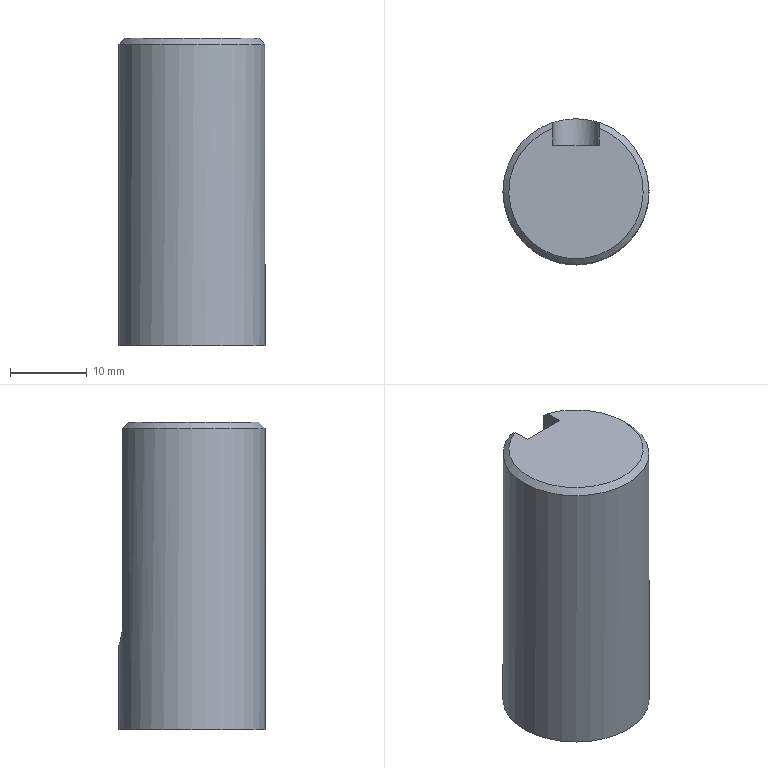Part | STEP file | Y2_SCZ_80_1.step 6 | 1 solid | 8 faces | box 19 x 19 x 40 mm | volume 10757 mm3 | plane 5 | cylinder 2 | cone 1 | commonest cylinder face diameters 6 x1 19 x1
STEP:
#1=CARTESIAN_POINT('',(0.,0.,0.));
#2=DIRECTION('',(0.,0.,1.));
#3=DIRECTION('',(1.,0.,0.));
#4=AXIS2_PLACEMENT_3D('',#1,#2,#3);
#5=CARTESIAN_POINT('',(3.,9.014,114.));
#6=VERTEX_POINT('',#5);
#7=CARTESIAN_POINT('',(3.,9.014,139.24));
#8=VERTEX_POINT('',#7);
#9=CARTESIAN_POINT('',(3.,9.014,100.));
#10=DIRECTION('',(0.,0.,1.));
#11=VECTOR('',#10,1.);
#12=LINE('',#9,#11);
#13=CARTESIAN_POINT('',(0.,0.,100.));
#14=DIRECTION('',(0.,0.,-1.));
#15=DIRECTION('',(-1.,0.,0.));
#16=AXIS2_PLACEMENT_3D('',#13,#14,#15);
#17=CYLINDRICAL_SURFACE('',#16,9.5);
#18=CARTESIAN_POINT('',(1.892,0.));
#19=DIRECTION('',(0.,-1.));
#20=VECTOR('',#19,1.);
#21=LINE('',#18,#20);
#22=(GEOMETRIC_REPRESENTATION_CONTEXT(2)PARAMETRIC_REPRESENTATION_CONTEXT()REPRESENTATION_CONTEXT('',''));
#23=DEFINITIONAL_REPRESENTATION('',(#21),#22);
#24=PCURVE('',#17,#23);
#25=CARTESIAN_POINT('',(3.,6.,140.));
#26=DIRECTION('',(1.,0.,0.));
#27=DIRECTION('',(0.,0.,-1.));
#28=AXIS2_PLACEMENT_3D('',#25,#26,#27);
#29=PLANE('',#28);
#30=CARTESIAN_POINT('',(40.,3.014));
#31=DIRECTION('',(-1.,0.));
#32=VECTOR('',#31,1.);
#33=LINE('',#30,#32);
#34=(GEOMETRIC_REPRESENTATION_CONTEXT(2)PARAMETRIC_REPRESENTATION_CONTEXT()REPRESENTATION_CONTEXT('',''));
#35=DEFINITIONAL_REPRESENTATION('',(#33),#34);
#36=PCURVE('',#29,#35);
#37=SURFACE_CURVE('',#12,(#24,#36),.PCURVE_S1.);
#38=EDGE_CURVE('',#6,#8,#37,.T.);
#39=ORIENTED_EDGE('',*,*,#38,.T.);
#40=CARTESIAN_POINT('',(-9.5,0.,139.24));
#41=VERTEX_POINT('',#40);
#42=CARTESIAN_POINT('',(0.,0.,139.24));
#43=DIRECTION('',(0.,0.,-1.));
#44=DIRECTION('',(-1.,0.,0.));
#45=AXIS2_PLACEMENT_3D('',#42,#43,#44);
#46=CIRCLE('',#45,9.5);
#47=CARTESIAN_POINT('',(0.,-39.24));
#48=DIRECTION('',(1.,0.));
#49=VECTOR('',#48,1.);
#50=LINE('',#47,#49);
#51=(GEOMETRIC_REPRESENTATION_CONTEXT(2)PARAMETRIC_REPRESENTATION_CONTEXT()REPRESENTATION_CONTEXT('',''));
#52=DEFINITIONAL_REPRESENTATION('',(#50),#51);
#53=PCURVE('',#17,#52);
#54=CARTESIAN_POINT('',(0.,0.,139.24));
#55=DIRECTION('',(0.,0.,-1.));
#56=DIRECTION('',(-1.,0.,0.));
#57=AXIS2_PLACEMENT_3D('',#54,#55,#56);
#58=CONICAL_SURFACE('',#57,9.5,0.7854);
#59=CARTESIAN_POINT('',(0.,0.));
#60=DIRECTION('',(1.,0.));
#61=VECTOR('',#60,1.);
#62=LINE('',#59,#61);
#63=(GEOMETRIC_REPRESENTATION_CONTEXT(2)PARAMETRIC_REPRESENTATION_CONTEXT()REPRESENTATION_CONTEXT('',''));
#64=DEFINITIONAL_REPRESENTATION('',(#62),#63);
#65=PCURVE('',#58,#64);
#66=SURFACE_CURVE('',#46,(#53,#65),.PCURVE_S1.);
#67=EDGE_CURVE('',#8,#41,#66,.T.);
#68=ORIENTED_EDGE('',*,*,#67,.T.);
#69=CARTESIAN_POINT('',(-9.5,0.,100.));
#70=VERTEX_POINT('',#69);
#71=CARTESIAN_POINT('',(-9.5,0.,139.24));
#72=CARTESIAN_POINT('',(-9.5,0.,100.));
#73=B_SPLINE_CURVE_WITH_KNOTS('',1,(#71,#72),.UNSPECIFIED.,.F.,.F.,(2,2),(-39.24,0.),.PIECEWISE_BEZIER_KNOTS.);
#74=CARTESIAN_POINT('',(6.283,0.));
#75=DIRECTION('',(0.,1.));
#76=VECTOR('',#75,1.);
#77=LINE('',#74,#76);
#78=(GEOMETRIC_REPRESENTATION_CONTEXT(2)PARAMETRIC_REPRESENTATION_CONTEXT()REPRESENTATION_CONTEXT('',''));
#79=DEFINITIONAL_REPRESENTATION('',(#77),#78);
#80=PCURVE('',#17,#79);
#81=CARTESIAN_POINT('',(0.,0.));
#82=DIRECTION('',(0.,1.));
#83=VECTOR('',#82,1.);
#84=LINE('',#81,#83);
#85=(GEOMETRIC_REPRESENTATION_CONTEXT(2)PARAMETRIC_REPRESENTATION_CONTEXT()REPRESENTATION_CONTEXT('',''));
#86=DEFINITIONAL_REPRESENTATION('',(#84),#85);
#87=PCURVE('',#17,#86);
#88=SEAM_CURVE('',#73,(#80,#87),.PCURVE_S1.);
#89=EDGE_CURVE('',#41,#70,#88,.T.);
#90=ORIENTED_EDGE('',*,*,#89,.T.);
#91=CARTESIAN_POINT('',(0.,0.,100.));
#92=DIRECTION('',(0.,0.,1.));
#93=DIRECTION('',(-1.,0.,0.));
#94=AXIS2_PLACEMENT_3D('',#91,#92,#93);
#95=CIRCLE('',#94,9.5);
#96=CARTESIAN_POINT('',(6.283,0.));
#97=DIRECTION('',(-1.,0.));
#98=VECTOR('',#97,1.);
#99=LINE('',#96,#98);
#100=(GEOMETRIC_REPRESENTATION_CONTEXT(2)PARAMETRIC_REPRESENTATION_CONTEXT()REPRESENTATION_CONTEXT('',''));
#101=DEFINITIONAL_REPRESENTATION('',(#99),#100);
#102=PCURVE('',#17,#101);
#103=CARTESIAN_POINT('',(0.,9.5,100.));
#104=DIRECTION('',(0.,0.,-1.));
#105=DIRECTION('',(-1.,0.,0.));
#106=AXIS2_PLACEMENT_3D('',#103,#104,#105);
#107=PLANE('',#106);
#108=CARTESIAN_POINT('',(9.5,-9.5));
#109=CARTESIAN_POINT('',(9.5,-25.954));
#110=CARTESIAN_POINT('',(-4.75,-17.727));
#111=CARTESIAN_POINT('',(-19.,-9.5));
#112=CARTESIAN_POINT('',(-4.75,-1.273));
#113=CARTESIAN_POINT('',(9.5,6.954));
#114=CARTESIAN_POINT('',(9.5,-9.5));
#115=(BOUNDED_CURVE()B_SPLINE_CURVE(2,(#108,#109,#110,#111,#112,#113,#114),.UNSPECIFIED.,.T.,.F.)B_SPLINE_CURVE_WITH_KNOTS((1,2,2,2,2,1),(-2.094,0.,2.094,4.189,6.283,8.378),.UNSPECIFIED.)CURVE()GEOMETRIC_REPRESENTATION_ITEM()RATIONAL_B_SPLINE_CURVE((1.,0.5,1.,0.5,1.,0.5,1.))REPRESENTATION_ITEM(''));
#116=(GEOMETRIC_REPRESENTATION_CONTEXT(2)PARAMETRIC_REPRESENTATION_CONTEXT()REPRESENTATION_CONTEXT('',''));
#117=DEFINITIONAL_REPRESENTATION('',(#115),#116);
#118=PCURVE('',#107,#117);
#119=SURFACE_CURVE('',#95,(#102,#118),.PCURVE_S1.);
#120=EDGE_CURVE('',#70,#70,#119,.T.);
#121=ORIENTED_EDGE('',*,*,#120,.T.);
#122=ORIENTED_EDGE('',*,*,#89,.F.);
#123=CARTESIAN_POINT('',(-3.,9.014,139.24));
#124=VERTEX_POINT('',#123);
#125=CARTESIAN_POINT('',(0.,0.,139.24));
#126=DIRECTION('',(0.,0.,-1.));
#127=DIRECTION('',(-1.,0.,0.));
#128=AXIS2_PLACEMENT_3D('',#125,#126,#127);
#129=CIRCLE('',#128,9.5);
#130=CARTESIAN_POINT('',(-6.283,-39.24));
#131=DIRECTION('',(1.,0.));
#132=VECTOR('',#131,1.);
#133=LINE('',#130,#132);
#134=(GEOMETRIC_REPRESENTATION_CONTEXT(2)PARAMETRIC_REPRESENTATION_CONTEXT()REPRESENTATION_CONTEXT('',''));
#135=DEFINITIONAL_REPRESENTATION('',(#133),#134);
#136=PCURVE('',#17,#135);
#137=CARTESIAN_POINT('',(0.,0.));
#138=DIRECTION('',(1.,0.));
#139=VECTOR('',#138,1.);
#140=LINE('',#137,#139);
#141=(GEOMETRIC_REPRESENTATION_CONTEXT(2)PARAMETRIC_REPRESENTATION_CONTEXT()REPRESENTATION_CONTEXT('',''));
#142=DEFINITIONAL_REPRESENTATION('',(#140),#141);
#143=PCURVE('',#58,#142);
#144=SURFACE_CURVE('',#129,(#136,#143),.PCURVE_S1.);
#145=EDGE_CURVE('',#41,#124,#144,.T.);
#146=ORIENTED_EDGE('',*,*,#145,.T.);
#147=CARTESIAN_POINT('',(-3.,9.014,114.));
#148=VERTEX_POINT('',#147);
#149=CARTESIAN_POINT('',(-3.,9.014,100.));
#150=DIRECTION('',(0.,0.,-1.));
#151=VECTOR('',#150,1.);
#152=LINE('',#149,#151);
#153=CARTESIAN_POINT('',(1.25,0.));
#154=DIRECTION('',(0.,1.));
#155=VECTOR('',#154,1.);
#156=LINE('',#153,#155);
#157=(GEOMETRIC_REPRESENTATION_CONTEXT(2)PARAMETRIC_REPRESENTATION_CONTEXT()REPRESENTATION_CONTEXT('',''));
#158=DEFINITIONAL_REPRESENTATION('',(#156),#157);
#159=PCURVE('',#17,#158);
#160=CARTESIAN_POINT('',(-3.,6.,140.));
#161=DIRECTION('',(-1.,0.,0.));
#162=DIRECTION('',(0.,0.,1.));
#163=AXIS2_PLACEMENT_3D('',#160,#161,#162);
#164=PLANE('',#163);
#165=CARTESIAN_POINT('',(-40.,3.014));
#166=DIRECTION('',(-1.,0.));
#167=VECTOR('',#166,1.);
#168=LINE('',#165,#167);
#169=(GEOMETRIC_REPRESENTATION_CONTEXT(2)PARAMETRIC_REPRESENTATION_CONTEXT()REPRESENTATION_CONTEXT('',''));
#170=DEFINITIONAL_REPRESENTATION('',(#168),#169);
#171=PCURVE('',#164,#170);
#172=SURFACE_CURVE('',#152,(#159,#171),.PCURVE_S1.);
#173=EDGE_CURVE('',#124,#148,#172,.T.);
#174=ORIENTED_EDGE('',*,*,#173,.T.);
#175=CARTESIAN_POINT('',(-3.,9.014,114.));
#176=CARTESIAN_POINT('',(-3.,9.014,113.8));
#177=CARTESIAN_POINT('',(-2.98,9.021,113.605));
#178=CARTESIAN_POINT('',(-2.903,9.046,113.22));
#179=CARTESIAN_POINT('',(-2.845,9.064,113.028));
#180=CARTESIAN_POINT('',(-2.694,9.11,112.666));
#181=CARTESIAN_POINT('',(-2.602,9.137,112.494));
#182=CARTESIAN_POINT('',(-2.385,9.197,112.169));
#183=CARTESIAN_POINT('',(-2.259,9.229,112.016));
#184=CARTESIAN_POINT('',(-1.847,9.323,111.604));
#185=CARTESIAN_POINT('',(-1.514,9.386,111.381));
#186=CARTESIAN_POINT('',(-0.9738,9.452,111.156));
#187=CARTESIAN_POINT('',(-0.7834,9.47,111.097));
#188=CARTESIAN_POINT('',(-0.3956,9.494,111.02));
#189=CARTESIAN_POINT('',(-0.2001,9.5,111.));
#190=CARTESIAN_POINT('',(0.194,9.5,111.));
#191=CARTESIAN_POINT('',(0.3942,9.494,111.02));
#192=CARTESIAN_POINT('',(0.78,9.47,111.097));
#193=CARTESIAN_POINT('',(0.9677,9.452,111.153));
#194=CARTESIAN_POINT('',(1.333,9.408,111.305));
#195=CARTESIAN_POINT('',(1.506,9.381,111.398));
#196=CARTESIAN_POINT('',(1.83,9.324,111.615));
#197=CARTESIAN_POINT('',(1.982,9.292,111.74));
#198=CARTESIAN_POINT('',(2.259,9.229,112.016));
#199=CARTESIAN_POINT('',(2.382,9.197,112.166));
#200=CARTESIAN_POINT('',(2.6,9.138,112.49));
#201=CARTESIAN_POINT('',(2.694,9.11,112.665));
#202=CARTESIAN_POINT('',(2.844,9.065,113.026));
#203=CARTESIAN_POINT('',(2.902,9.046,113.213));
#204=CARTESIAN_POINT('',(2.98,9.021,113.601));
#205=CARTESIAN_POINT('',(3.,9.014,113.8));
#206=CARTESIAN_POINT('',(3.,9.014,114.));
#207=B_SPLINE_CURVE_WITH_KNOTS('',3,(#175,#176,#177,#178,#179,#180,#181,#182,#183,#184,#185,#186,#187,#188,#189,#190,#191,#192,#193,#194,#195,#196,#197,#198,#199,#200,#201,#202,#203,#204,#205,#206),.UNSPECIFIED.,.F.,.F.,(4,2,2,2,2,2,2,2,2,2,2,2,2,2,2,4),(0.,0.0005898,0.00118,0.001769,0.002359,0.003539,0.004128,0.004718,0.005308,0.005898,0.006488,0.007077,0.007667,0.008257,0.008847,0.009437),.UNSPECIFIED.);
#208=CARTESIAN_POINT('',(1.25,-14.));
#209=CARTESIAN_POINT('',(1.25,-13.952));
#210=CARTESIAN_POINT('',(1.25,-13.855));
#211=CARTESIAN_POINT('',(1.251,-13.712));
#212=CARTESIAN_POINT('',(1.253,-13.57));
#213=CARTESIAN_POINT('',(1.255,-13.429));
#214=CARTESIAN_POINT('',(1.259,-13.29));
#215=CARTESIAN_POINT('',(1.263,-13.151));
#216=CARTESIAN_POINT('',(1.268,-13.014));
#217=CARTESIAN_POINT('',(1.273,-12.88));
#218=CARTESIAN_POINT('',(1.28,-12.749));
#219=CARTESIAN_POINT('',(1.286,-12.621));
#220=CARTESIAN_POINT('',(1.294,-12.497));
#221=CARTESIAN_POINT('',(1.302,-12.376));
#222=CARTESIAN_POINT('',(1.311,-12.258));
#223=CARTESIAN_POINT('',(1.32,-12.144));
#224=CARTESIAN_POINT('',(1.33,-12.034));
#225=CARTESIAN_POINT('',(1.34,-11.929));
#226=CARTESIAN_POINT('',(1.351,-11.829));
#227=CARTESIAN_POINT('',(1.362,-11.733));
#228=CARTESIAN_POINT('',(1.374,-11.643));
#229=CARTESIAN_POINT('',(1.386,-11.558));
#230=CARTESIAN_POINT('',(1.399,-11.478));
#231=CARTESIAN_POINT('',(1.412,-11.404));
#232=CARTESIAN_POINT('',(1.425,-11.335));
#233=CARTESIAN_POINT('',(1.439,-11.273));
#234=CARTESIAN_POINT('',(1.452,-11.216));
#235=CARTESIAN_POINT('',(1.467,-11.166));
#236=CARTESIAN_POINT('',(1.481,-11.122));
#237=CARTESIAN_POINT('',(1.496,-11.085));
#238=CARTESIAN_POINT('',(1.511,-11.054));
#239=CARTESIAN_POINT('',(1.525,-11.03));
#240=CARTESIAN_POINT('',(1.54,-11.013));
#241=CARTESIAN_POINT('',(1.555,-11.002));
#242=CARTESIAN_POINT('',(1.57,-10.999));
#243=CARTESIAN_POINT('',(1.586,-11.002));
#244=CARTESIAN_POINT('',(1.601,-11.012));
#245=CARTESIAN_POINT('',(1.616,-11.03));
#246=CARTESIAN_POINT('',(1.631,-11.053));
#247=CARTESIAN_POINT('',(1.646,-11.084));
#248=CARTESIAN_POINT('',(1.66,-11.121));
#249=CARTESIAN_POINT('',(1.674,-11.164));
#250=CARTESIAN_POINT('',(1.689,-11.215));
#251=CARTESIAN_POINT('',(1.703,-11.271));
#252=CARTESIAN_POINT('',(1.716,-11.334));
#253=CARTESIAN_POINT('',(1.73,-11.402));
#254=CARTESIAN_POINT('',(1.743,-11.476));
#255=CARTESIAN_POINT('',(1.755,-11.556));
#256=CARTESIAN_POINT('',(1.767,-11.641));
#257=CARTESIAN_POINT('',(1.779,-11.732));
#258=CARTESIAN_POINT('',(1.791,-11.828));
#259=CARTESIAN_POINT('',(1.801,-11.928));
#260=CARTESIAN_POINT('',(1.812,-12.033));
#261=CARTESIAN_POINT('',(1.821,-12.142));
#262=CARTESIAN_POINT('',(1.831,-12.255));
#263=CARTESIAN_POINT('',(1.839,-12.372));
#264=CARTESIAN_POINT('',(1.848,-12.494));
#265=CARTESIAN_POINT('',(1.855,-12.619));
#266=CARTESIAN_POINT('',(1.862,-12.748));
#267=CARTESIAN_POINT('',(1.868,-12.878));
#268=CARTESIAN_POINT('',(1.874,-13.011));
#269=CARTESIAN_POINT('',(1.879,-13.147));
#270=CARTESIAN_POINT('',(1.883,-13.284));
#271=CARTESIAN_POINT('',(1.886,-13.425));
#272=CARTESIAN_POINT('',(1.889,-13.567));
#273=CARTESIAN_POINT('',(1.891,-13.71));
#274=CARTESIAN_POINT('',(1.892,-13.855));
#275=CARTESIAN_POINT('',(1.892,-13.952));
#276=CARTESIAN_POINT('',(1.892,-14.));
#277=B_SPLINE_CURVE_WITH_KNOTS('',3,(#208,#209,#210,#211,#212,#213,#214,#215,#216,#217,#218,#219,#220,#221,#222,#223,#224,#225,#226,#227,#228,#229,#230,#231,#232,#233,#234,#235,#236,#237,#238,#239,#240,#241,#242,#243,#244,#245,#246,#247,#248,#249,#250,#251,#252,#253,#254,#255,#256,#257,#258,#259,#260,#261,#262,#263,#264,#265,#266,#267,#268,#269,#270,#271,#272,#273,#274,#275,#276),.UNSPECIFIED.,.F.,.F.,(4,1,1,1,1,1,1,1,1,1,1,1,1,1,1,1,1,1,1,1,1,1,1,1,1,1,1,1,1,1,1,1,1,1,1,1,1,1,1,1,1,1,1,1,1,1,1,1,1,1,1,1,1,1,1,1,1,1,1,1,1,1,1,1,1,1,4),(0.,0.000143,0.000286,0.0004289,0.0005719,0.0007149,0.0008579,0.001001,0.001144,0.001287,0.00143,0.001573,0.001716,0.001859,0.002002,0.002145,0.002288,0.002431,0.002574,0.002717,0.00286,0.003003,0.003146,0.003288,0.003431,0.003574,0.003717,0.00386,0.004003,0.004146,0.004289,0.004432,0.004575,0.004718,0.004861,0.005004,0.005147,0.00529,0.005433,0.005576,0.005719,0.005862,0.006005,0.006148,0.006291,0.006434,0.006577,0.00672,0.006863,0.007006,0.007149,0.007292,0.007435,0.007578,0.007721,0.007864,0.008007,0.00815,0.008293,0.008436,0.008579,0.008722,0.008865,0.009008,0.009151,0.009294,0.009437),.QUASI_UNIFORM_KNOTS.);
#278=(GEOMETRIC_REPRESENTATION_CONTEXT(2)PARAMETRIC_REPRESENTATION_CONTEXT()REPRESENTATION_CONTEXT('',''));
#279=DEFINITIONAL_REPRESENTATION('',(#277),#278);
#280=PCURVE('',#17,#279);
#281=CARTESIAN_POINT('',(0.,6.,114.));
#282=DIRECTION('',(0.,1.,0.));
#283=DIRECTION('',(0.,0.,1.));
#284=AXIS2_PLACEMENT_3D('',#281,#282,#283);
#285=CYLINDRICAL_SURFACE('',#284,3.);
#286=CARTESIAN_POINT('',(4.712,3.014));
#287=CARTESIAN_POINT('',(4.696,3.014));
#288=CARTESIAN_POINT('',(4.664,3.015));
#289=CARTESIAN_POINT('',(4.616,3.018));
#290=CARTESIAN_POINT('',(4.569,3.024));
#291=CARTESIAN_POINT('',(4.521,3.032));
#292=CARTESIAN_POINT('',(4.473,3.041));
#293=CARTESIAN_POINT('',(4.426,3.053));
#294=CARTESIAN_POINT('',(4.378,3.067));
#295=CARTESIAN_POINT('',(4.33,3.083));
#296=CARTESIAN_POINT('',(4.282,3.1));
#297=CARTESIAN_POINT('',(4.235,3.118));
#298=CARTESIAN_POINT('',(4.188,3.138));
#299=CARTESIAN_POINT('',(4.14,3.159));
#300=CARTESIAN_POINT('',(4.093,3.18));
#301=CARTESIAN_POINT('',(4.045,3.203));
#302=CARTESIAN_POINT('',(3.998,3.226));
#303=CARTESIAN_POINT('',(3.951,3.249));
#304=CARTESIAN_POINT('',(3.904,3.272));
#305=CARTESIAN_POINT('',(3.856,3.294));
#306=CARTESIAN_POINT('',(3.809,3.317));
#307=CARTESIAN_POINT('',(3.762,3.339));
#308=CARTESIAN_POINT('',(3.714,3.36));
#309=CARTESIAN_POINT('',(3.667,3.38));
#310=CARTESIAN_POINT('',(3.619,3.399));
#311=CARTESIAN_POINT('',(3.572,3.417));
#312=CARTESIAN_POINT('',(3.525,3.434));
#313=CARTESIAN_POINT('',(3.477,3.449));
#314=CARTESIAN_POINT('',(3.429,3.462));
#315=CARTESIAN_POINT('',(3.381,3.474));
#316=CARTESIAN_POINT('',(3.333,3.483));
#317=CARTESIAN_POINT('',(3.286,3.491));
#318=CARTESIAN_POINT('',(3.238,3.496));
#319=CARTESIAN_POINT('',(3.19,3.499));
#320=CARTESIAN_POINT('',(3.143,3.5));
#321=CARTESIAN_POINT('',(3.095,3.499));
#322=CARTESIAN_POINT('',(3.047,3.496));
#323=CARTESIAN_POINT('',(2.998,3.491));
#324=CARTESIAN_POINT('',(2.951,3.483));
#325=CARTESIAN_POINT('',(2.903,3.474));
#326=CARTESIAN_POINT('',(2.855,3.462));
#327=CARTESIAN_POINT('',(2.808,3.449));
#328=CARTESIAN_POINT('',(2.76,3.434));
#329=CARTESIAN_POINT('',(2.712,3.418));
#330=CARTESIAN_POINT('',(2.665,3.4));
#331=CARTESIAN_POINT('',(2.617,3.381));
#332=CARTESIAN_POINT('',(2.57,3.36));
#333=CARTESIAN_POINT('',(2.523,3.339));
#334=CARTESIAN_POINT('',(2.475,3.317));
#335=CARTESIAN_POINT('',(2.428,3.295));
#336=CARTESIAN_POINT('',(2.38,3.272));
#337=CARTESIAN_POINT('',(2.333,3.249));
#338=CARTESIAN_POINT('',(2.286,3.226));
#339=CARTESIAN_POINT('',(2.239,3.203));
#340=CARTESIAN_POINT('',(2.191,3.181));
#341=CARTESIAN_POINT('',(2.144,3.159));
#342=CARTESIAN_POINT('',(2.097,3.139));
#343=CARTESIAN_POINT('',(2.049,3.119));
#344=CARTESIAN_POINT('',(2.001,3.1));
#345=CARTESIAN_POINT('',(1.954,3.083));
#346=CARTESIAN_POINT('',(1.906,3.068));
#347=CARTESIAN_POINT('',(1.859,3.054));
#348=CARTESIAN_POINT('',(1.812,3.042));
#349=CARTESIAN_POINT('',(1.764,3.032));
#350=CARTESIAN_POINT('',(1.716,3.024));
#351=CARTESIAN_POINT('',(1.667,3.018));
#352=CARTESIAN_POINT('',(1.619,3.015));
#353=CARTESIAN_POINT('',(1.587,3.014));
#354=CARTESIAN_POINT('',(1.571,3.014));
#355=B_SPLINE_CURVE_WITH_KNOTS('',3,(#286,#287,#288,#289,#290,#291,#292,#293,#294,#295,#296,#297,#298,#299,#300,#301,#302,#303,#304,#305,#306,#307,#308,#309,#310,#311,#312,#313,#314,#315,#316,#317,#318,#319,#320,#321,#322,#323,#324,#325,#326,#327,#328,#329,#330,#331,#332,#333,#334,#335,#336,#337,#338,#339,#340,#341,#342,#343,#344,#345,#346,#347,#348,#349,#350,#351,#352,#353,#354),.UNSPECIFIED.,.F.,.F.,(4,1,1,1,1,1,1,1,1,1,1,1,1,1,1,1,1,1,1,1,1,1,1,1,1,1,1,1,1,1,1,1,1,1,1,1,1,1,1,1,1,1,1,1,1,1,1,1,1,1,1,1,1,1,1,1,1,1,1,1,1,1,1,1,1,1,4),(0.,0.000143,0.000286,0.0004289,0.0005719,0.0007149,0.0008579,0.001001,0.001144,0.001287,0.00143,0.001573,0.001716,0.001859,0.002002,0.002145,0.002288,0.002431,0.002574,0.002717,0.00286,0.003003,0.003146,0.003288,0.003431,0.003574,0.003717,0.00386,0.004003,0.004146,0.004289,0.004432,0.004575,0.004718,0.004861,0.005004,0.005147,0.00529,0.005433,0.005576,0.005719,0.005862,0.006005,0.006148,0.006291,0.006434,0.006577,0.00672,0.006863,0.007006,0.007149,0.007292,0.007435,0.007578,0.007721,0.007864,0.008007,0.00815,0.008293,0.008436,0.008579,0.008722,0.008865,0.009008,0.009151,0.009294,0.009437),.QUASI_UNIFORM_KNOTS.);
#356=(GEOMETRIC_REPRESENTATION_CONTEXT(2)PARAMETRIC_REPRESENTATION_CONTEXT()REPRESENTATION_CONTEXT('',''));
#357=DEFINITIONAL_REPRESENTATION('',(#355),#356);
#358=PCURVE('',#285,#357);
#359=SURFACE_CURVE('',#207,(#280,#358),.PCURVE_S1.);
#360=EDGE_CURVE('',#148,#6,#359,.T.);
#361=ORIENTED_EDGE('',*,*,#360,.T.);
#362=EDGE_LOOP('',(#39,#68,#90,#121,#122,#146,#174,#361));
#363=FACE_BOUND('',#362,.T.);
#364=ADVANCED_FACE('',(#363),#17,.T.);
#365=ORIENTED_EDGE('',*,*,#120,.F.);
#366=EDGE_LOOP('',(#365));
#367=FACE_BOUND('',#366,.T.);
#368=ADVANCED_FACE('',(#367),#107,.T.);
#369=CARTESIAN_POINT('',(3.,8.209,140.));
#370=VERTEX_POINT('',#369);
#371=CARTESIAN_POINT('',(-3.,8.209,140.));
#372=VERTEX_POINT('',#371);
#373=CARTESIAN_POINT('',(0.,0.,140.));
#374=DIRECTION('',(0.,0.,-1.));
#375=DIRECTION('',(-1.,0.,0.));
#376=AXIS2_PLACEMENT_3D('',#373,#374,#375);
#377=CIRCLE('',#376,8.74);
#378=CARTESIAN_POINT('',(0.,-0.76));
#379=DIRECTION('',(1.,0.));
#380=VECTOR('',#379,1.);
#381=LINE('',#378,#380);
#382=(GEOMETRIC_REPRESENTATION_CONTEXT(2)PARAMETRIC_REPRESENTATION_CONTEXT()REPRESENTATION_CONTEXT('',''));
#383=DEFINITIONAL_REPRESENTATION('',(#381),#382);
#384=PCURVE('',#58,#383);
#385=CARTESIAN_POINT('',(0.,0.,140.));
#386=DIRECTION('',(0.,0.,1.));
#387=DIRECTION('',(1.,0.,0.));
#388=AXIS2_PLACEMENT_3D('',#385,#386,#387);
#389=PLANE('',#388);
#390=CARTESIAN_POINT('',(-8.74,0.));
#391=CARTESIAN_POINT('',(-8.74,15.138));
#392=CARTESIAN_POINT('',(4.37,7.569));
#393=CARTESIAN_POINT('',(17.48,0.));
#394=CARTESIAN_POINT('',(4.37,-7.569));
#395=CARTESIAN_POINT('',(-8.74,-15.138));
#396=CARTESIAN_POINT('',(-8.74,0.));
#397=(BOUNDED_CURVE()B_SPLINE_CURVE(2,(#390,#391,#392,#393,#394,#395,#396),.UNSPECIFIED.,.T.,.F.)B_SPLINE_CURVE_WITH_KNOTS((1,2,2,2,2,1),(-2.094,0.,2.094,4.189,6.283,8.378),.UNSPECIFIED.)CURVE()GEOMETRIC_REPRESENTATION_ITEM()RATIONAL_B_SPLINE_CURVE((1.,0.5,1.,0.5,1.,0.5,1.))REPRESENTATION_ITEM(''));
#398=(GEOMETRIC_REPRESENTATION_CONTEXT(2)PARAMETRIC_REPRESENTATION_CONTEXT()REPRESENTATION_CONTEXT('',''));
#399=DEFINITIONAL_REPRESENTATION('',(#397),#398);
#400=PCURVE('',#389,#399);
#401=SURFACE_CURVE('',#377,(#384,#400),.PCURVE_S1.);
#402=EDGE_CURVE('',#370,#372,#401,.T.);
#403=ORIENTED_EDGE('',*,*,#402,.T.);
#404=CARTESIAN_POINT('',(-3.,8.209,140.));
#405=CARTESIAN_POINT('',(-3.,8.478,139.747));
#406=CARTESIAN_POINT('',(-3.,8.746,139.494));
#407=CARTESIAN_POINT('',(-3.,9.014,139.24));
#408=B_SPLINE_CURVE_WITH_KNOTS('',3,(#404,#405,#406,#407),.UNSPECIFIED.,.F.,.F.,(4,4),(0.,0.001107),.PIECEWISE_BEZIER_KNOTS.);
#409=CARTESIAN_POINT('',(7.504,-0.76));
#410=CARTESIAN_POINT('',(7.504,-0.7485));
#411=CARTESIAN_POINT('',(7.505,-0.7255));
#412=CARTESIAN_POINT('',(7.506,-0.6911));
#413=CARTESIAN_POINT('',(7.508,-0.6566));
#414=CARTESIAN_POINT('',(7.509,-0.6221));
#415=CARTESIAN_POINT('',(7.511,-0.5876));
#416=CARTESIAN_POINT('',(7.512,-0.5531));
#417=CARTESIAN_POINT('',(7.513,-0.5186));
#418=CARTESIAN_POINT('',(7.515,-0.4841));
#419=CARTESIAN_POINT('',(7.516,-0.4496));
#420=CARTESIAN_POINT('',(7.517,-0.4151));
#421=CARTESIAN_POINT('',(7.519,-0.3805));
#422=CARTESIAN_POINT('',(7.52,-0.346));
#423=CARTESIAN_POINT('',(7.521,-0.3114));
#424=CARTESIAN_POINT('',(7.523,-0.2768));
#425=CARTESIAN_POINT('',(7.524,-0.2423));
#426=CARTESIAN_POINT('',(7.525,-0.2077));
#427=CARTESIAN_POINT('',(7.527,-0.1731));
#428=CARTESIAN_POINT('',(7.528,-0.1385));
#429=CARTESIAN_POINT('',(7.529,-0.1039));
#430=CARTESIAN_POINT('',(7.53,-0.06925));
#431=CARTESIAN_POINT('',(7.531,-0.03463));
#432=CARTESIAN_POINT('',(7.532,-0.01154));
#433=CARTESIAN_POINT('',(7.533,0.));
#434=B_SPLINE_CURVE_WITH_KNOTS('',3,(#409,#410,#411,#412,#413,#414,#415,#416,#417,#418,#419,#420,#421,#422,#423,#424,#425,#426,#427,#428,#429,#430,#431,#432,#433),.UNSPECIFIED.,.F.,.F.,(4,1,1,1,1,1,1,1,1,1,1,1,1,1,1,1,1,1,1,1,1,1,4),(0.,0.00005032,0.0001006,0.000151,0.0002013,0.0002516,0.0003019,0.0003522,0.0004025,0.0004529,0.0005032,0.0005535,0.0006038,0.0006541,0.0007045,0.0007548,0.0008051,0.0008554,0.0009057,0.000956,0.001006,0.001057,0.001107),.QUASI_UNIFORM_KNOTS.);
#435=(GEOMETRIC_REPRESENTATION_CONTEXT(2)PARAMETRIC_REPRESENTATION_CONTEXT()REPRESENTATION_CONTEXT('',''));
#436=DEFINITIONAL_REPRESENTATION('',(#434),#435);
#437=PCURVE('',#58,#436);
#438=CARTESIAN_POINT('',(0.,2.209));
#439=CARTESIAN_POINT('',(-0.2526,2.478));
#440=CARTESIAN_POINT('',(-0.506,2.746));
#441=CARTESIAN_POINT('',(-0.76,3.014));
#442=B_SPLINE_CURVE_WITH_KNOTS('',3,(#438,#439,#440,#441),.UNSPECIFIED.,.F.,.F.,(4,4),(0.,0.001107),.PIECEWISE_BEZIER_KNOTS.);
#443=(GEOMETRIC_REPRESENTATION_CONTEXT(2)PARAMETRIC_REPRESENTATION_CONTEXT()REPRESENTATION_CONTEXT('',''));
#444=DEFINITIONAL_REPRESENTATION('',(#442),#443);
#445=PCURVE('',#164,#444);
#446=SURFACE_CURVE('',#408,(#437,#445),.PCURVE_S1.);
#447=EDGE_CURVE('',#372,#124,#446,.T.);
#448=ORIENTED_EDGE('',*,*,#447,.T.);
#449=ORIENTED_EDGE('',*,*,#145,.F.);
#450=ORIENTED_EDGE('',*,*,#67,.F.);
#451=CARTESIAN_POINT('',(3.,9.014,139.24));
#452=CARTESIAN_POINT('',(3.,8.746,139.494));
#453=CARTESIAN_POINT('',(3.,8.478,139.747));
#454=CARTESIAN_POINT('',(3.,8.209,140.));
#455=B_SPLINE_CURVE_WITH_KNOTS('',3,(#451,#452,#453,#454),.UNSPECIFIED.,.F.,.F.,(4,4),(0.,0.001107),.PIECEWISE_BEZIER_KNOTS.);
#456=CARTESIAN_POINT('',(1.892,0.));
#457=CARTESIAN_POINT('',(1.892,-0.01154));
#458=CARTESIAN_POINT('',(1.893,-0.03463));
#459=CARTESIAN_POINT('',(1.895,-0.06925));
#460=CARTESIAN_POINT('',(1.896,-0.1039));
#461=CARTESIAN_POINT('',(1.897,-0.1385));
#462=CARTESIAN_POINT('',(1.898,-0.1731));
#463=CARTESIAN_POINT('',(1.9,-0.2077));
#464=CARTESIAN_POINT('',(1.901,-0.2423));
#465=CARTESIAN_POINT('',(1.902,-0.2768));
#466=CARTESIAN_POINT('',(1.903,-0.3114));
#467=CARTESIAN_POINT('',(1.905,-0.346));
#468=CARTESIAN_POINT('',(1.906,-0.3805));
#469=CARTESIAN_POINT('',(1.907,-0.4151));
#470=CARTESIAN_POINT('',(1.909,-0.4496));
#471=CARTESIAN_POINT('',(1.91,-0.4841));
#472=CARTESIAN_POINT('',(1.911,-0.5186));
#473=CARTESIAN_POINT('',(1.913,-0.5531));
#474=CARTESIAN_POINT('',(1.914,-0.5876));
#475=CARTESIAN_POINT('',(1.915,-0.6221));
#476=CARTESIAN_POINT('',(1.917,-0.6566));
#477=CARTESIAN_POINT('',(1.918,-0.6911));
#478=CARTESIAN_POINT('',(1.92,-0.7255));
#479=CARTESIAN_POINT('',(1.921,-0.7485));
#480=CARTESIAN_POINT('',(1.921,-0.76));
#481=B_SPLINE_CURVE_WITH_KNOTS('',3,(#456,#457,#458,#459,#460,#461,#462,#463,#464,#465,#466,#467,#468,#469,#470,#471,#472,#473,#474,#475,#476,#477,#478,#479,#480),.UNSPECIFIED.,.F.,.F.,(4,1,1,1,1,1,1,1,1,1,1,1,1,1,1,1,1,1,1,1,1,1,4),(0.,0.00005032,0.0001006,0.000151,0.0002013,0.0002516,0.0003019,0.0003522,0.0004025,0.0004529,0.0005032,0.0005535,0.0006038,0.0006541,0.0007045,0.0007548,0.0008051,0.0008554,0.0009057,0.000956,0.001006,0.001057,0.001107),.QUASI_UNIFORM_KNOTS.);
#482=(GEOMETRIC_REPRESENTATION_CONTEXT(2)PARAMETRIC_REPRESENTATION_CONTEXT()REPRESENTATION_CONTEXT('',''));
#483=DEFINITIONAL_REPRESENTATION('',(#481),#482);
#484=PCURVE('',#58,#483);
#485=CARTESIAN_POINT('',(0.76,3.014));
#486=CARTESIAN_POINT('',(0.506,2.746));
#487=CARTESIAN_POINT('',(0.2526,2.478));
#488=CARTESIAN_POINT('',(0.,2.209));
#489=B_SPLINE_CURVE_WITH_KNOTS('',3,(#485,#486,#487,#488),.UNSPECIFIED.,.F.,.F.,(4,4),(0.,0.001107),.PIECEWISE_BEZIER_KNOTS.);
#490=(GEOMETRIC_REPRESENTATION_CONTEXT(2)PARAMETRIC_REPRESENTATION_CONTEXT()REPRESENTATION_CONTEXT('',''));
#491=DEFINITIONAL_REPRESENTATION('',(#489),#490);
#492=PCURVE('',#29,#491);
#493=SURFACE_CURVE('',#455,(#484,#492),.PCURVE_S1.);
#494=EDGE_CURVE('',#8,#370,#493,.T.);
#495=ORIENTED_EDGE('',*,*,#494,.T.);
#496=EDGE_LOOP('',(#403,#448,#449,#450,#495));
#497=FACE_BOUND('',#496,.T.);
#498=ADVANCED_FACE('',(#497),#58,.T.);
#499=CARTESIAN_POINT('',(3.,6.,114.));
#500=VERTEX_POINT('',#499);
#501=CARTESIAN_POINT('',(3.,6.,114.));
#502=DIRECTION('',(0.,1.,0.));
#503=VECTOR('',#502,1.);
#504=LINE('',#501,#503);
#505=CARTESIAN_POINT('',(26.,0.));
#506=DIRECTION('',(0.,1.));
#507=VECTOR('',#506,1.);
#508=LINE('',#505,#507);
#509=(GEOMETRIC_REPRESENTATION_CONTEXT(2)PARAMETRIC_REPRESENTATION_CONTEXT()REPRESENTATION_CONTEXT('',''));
#510=DEFINITIONAL_REPRESENTATION('',(#508),#509);
#511=PCURVE('',#29,#510);
#512=CARTESIAN_POINT('',(1.571,0.));
#513=DIRECTION('',(0.,1.));
#514=VECTOR('',#513,1.);
#515=LINE('',#512,#514);
#516=(GEOMETRIC_REPRESENTATION_CONTEXT(2)PARAMETRIC_REPRESENTATION_CONTEXT()REPRESENTATION_CONTEXT('',''));
#517=DEFINITIONAL_REPRESENTATION('',(#515),#516);
#518=PCURVE('',#285,#517);
#519=SURFACE_CURVE('',#504,(#511,#518),.PCURVE_S1.);
#520=EDGE_CURVE('',#500,#6,#519,.T.);
#521=ORIENTED_EDGE('',*,*,#520,.F.);
#522=CARTESIAN_POINT('',(3.,6.,140.));
#523=VERTEX_POINT('',#522);
#524=CARTESIAN_POINT('',(3.,6.,140.));
#525=DIRECTION('',(0.,0.,-1.));
#526=VECTOR('',#525,1.);
#527=LINE('',#524,#526);
#528=CARTESIAN_POINT('',(0.,0.));
#529=DIRECTION('',(1.,0.));
#530=VECTOR('',#529,1.);
#531=LINE('',#528,#530);
#532=(GEOMETRIC_REPRESENTATION_CONTEXT(2)PARAMETRIC_REPRESENTATION_CONTEXT()REPRESENTATION_CONTEXT('',''));
#533=DEFINITIONAL_REPRESENTATION('',(#531),#532);
#534=PCURVE('',#29,#533);
#535=CARTESIAN_POINT('',(0.,6.,114.));
#536=DIRECTION('',(0.,1.,0.));
#537=DIRECTION('',(0.,0.,1.));
#538=AXIS2_PLACEMENT_3D('',#535,#536,#537);
#539=PLANE('',#538);
#540=CARTESIAN_POINT('',(26.,3.));
#541=DIRECTION('',(-1.,0.));
#542=VECTOR('',#541,1.);
#543=LINE('',#540,#542);
#544=(GEOMETRIC_REPRESENTATION_CONTEXT(2)PARAMETRIC_REPRESENTATION_CONTEXT()REPRESENTATION_CONTEXT('',''));
#545=DEFINITIONAL_REPRESENTATION('',(#543),#544);
#546=PCURVE('',#539,#545);
#547=SURFACE_CURVE('',#527,(#534,#546),.PCURVE_S1.);
#548=EDGE_CURVE('',#523,#500,#547,.T.);
#549=ORIENTED_EDGE('',*,*,#548,.F.);
#550=CARTESIAN_POINT('',(3.,6.,140.));
#551=DIRECTION('',(0.,-1.,0.));
#552=VECTOR('',#551,1.);
#553=LINE('',#550,#552);
#554=CARTESIAN_POINT('',(0.,0.));
#555=DIRECTION('',(0.,-1.));
#556=VECTOR('',#555,1.);
#557=LINE('',#554,#556);
#558=(GEOMETRIC_REPRESENTATION_CONTEXT(2)PARAMETRIC_REPRESENTATION_CONTEXT()REPRESENTATION_CONTEXT('',''));
#559=DEFINITIONAL_REPRESENTATION('',(#557),#558);
#560=PCURVE('',#29,#559);
#561=CARTESIAN_POINT('',(3.,6.));
#562=DIRECTION('',(0.,-1.));
#563=VECTOR('',#562,1.);
#564=LINE('',#561,#563);
#565=(GEOMETRIC_REPRESENTATION_CONTEXT(2)PARAMETRIC_REPRESENTATION_CONTEXT()REPRESENTATION_CONTEXT('',''));
#566=DEFINITIONAL_REPRESENTATION('',(#564),#565);
#567=PCURVE('',#389,#566);
#568=SURFACE_CURVE('',#553,(#560,#567),.PCURVE_S1.);
#569=EDGE_CURVE('',#370,#523,#568,.T.);
#570=ORIENTED_EDGE('',*,*,#569,.F.);
#571=ORIENTED_EDGE('',*,*,#494,.F.);
#572=ORIENTED_EDGE('',*,*,#38,.F.);
#573=EDGE_LOOP('',(#521,#549,#570,#571,#572));
#574=FACE_BOUND('',#573,.T.);
#575=ADVANCED_FACE('',(#574),#29,.F.);
#576=ORIENTED_EDGE('',*,*,#360,.T.);
#577=ORIENTED_EDGE('',*,*,#520,.F.);
#578=CARTESIAN_POINT('',(-3.,6.,114.));
#579=VERTEX_POINT('',#578);
#580=CARTESIAN_POINT('',(0.,6.,114.));
#581=DIRECTION('',(0.,1.,0.));
#582=DIRECTION('',(0.,0.,1.));
#583=AXIS2_PLACEMENT_3D('',#580,#581,#582);
#584=CIRCLE('',#583,3.);
#585=CARTESIAN_POINT('',(0.,0.));
#586=DIRECTION('',(1.,0.));
#587=VECTOR('',#586,1.);
#588=LINE('',#585,#587);
#589=(GEOMETRIC_REPRESENTATION_CONTEXT(2)PARAMETRIC_REPRESENTATION_CONTEXT()REPRESENTATION_CONTEXT('',''));
#590=DEFINITIONAL_REPRESENTATION('',(#588),#589);
#591=PCURVE('',#285,#590);
#592=CARTESIAN_POINT('',(0.,0.));
#593=DIRECTION('',(1.,0.));
#594=AXIS2_PLACEMENT_2D('',#592,#593);
#595=CIRCLE('',#594,3.);
#596=(GEOMETRIC_REPRESENTATION_CONTEXT(2)PARAMETRIC_REPRESENTATION_CONTEXT()REPRESENTATION_CONTEXT('',''));
#597=DEFINITIONAL_REPRESENTATION('',(#595),#596);
#598=PCURVE('',#539,#597);
#599=SURFACE_CURVE('',#584,(#591,#598),.PCURVE_S1.);
#600=EDGE_CURVE('',#500,#579,#599,.T.);
#601=ORIENTED_EDGE('',*,*,#600,.T.);
#602=CARTESIAN_POINT('',(-3.,6.,114.));
#603=DIRECTION('',(0.,1.,0.));
#604=VECTOR('',#603,1.);
#605=LINE('',#602,#604);
#606=CARTESIAN_POINT('',(4.712,0.));
#607=DIRECTION('',(0.,1.));
#608=VECTOR('',#607,1.);
#609=LINE('',#606,#608);
#610=(GEOMETRIC_REPRESENTATION_CONTEXT(2)PARAMETRIC_REPRESENTATION_CONTEXT()REPRESENTATION_CONTEXT('',''));
#611=DEFINITIONAL_REPRESENTATION('',(#609),#610);
#612=PCURVE('',#285,#611);
#613=CARTESIAN_POINT('',(-26.,0.));
#614=DIRECTION('',(0.,1.));
#615=VECTOR('',#614,1.);
#616=LINE('',#613,#615);
#617=(GEOMETRIC_REPRESENTATION_CONTEXT(2)PARAMETRIC_REPRESENTATION_CONTEXT()REPRESENTATION_CONTEXT('',''));
#618=DEFINITIONAL_REPRESENTATION('',(#616),#617);
#619=PCURVE('',#164,#618);
#620=SURFACE_CURVE('',#605,(#612,#619),.PCURVE_S1.);
#621=EDGE_CURVE('',#579,#148,#620,.T.);
#622=ORIENTED_EDGE('',*,*,#621,.T.);
#623=EDGE_LOOP('',(#576,#577,#601,#622));
#624=FACE_BOUND('',#623,.F.);
#625=ADVANCED_FACE('',(#624),#285,.F.);
#626=ORIENTED_EDGE('',*,*,#447,.F.);
#627=CARTESIAN_POINT('',(-3.,6.,140.));
#628=VERTEX_POINT('',#627);
#629=CARTESIAN_POINT('',(-3.,6.,140.));
#630=DIRECTION('',(0.,1.,0.));
#631=VECTOR('',#630,1.);
#632=LINE('',#629,#631);
#633=CARTESIAN_POINT('',(0.,0.));
#634=DIRECTION('',(0.,1.));
#635=VECTOR('',#634,1.);
#636=LINE('',#633,#635);
#637=(GEOMETRIC_REPRESENTATION_CONTEXT(2)PARAMETRIC_REPRESENTATION_CONTEXT()REPRESENTATION_CONTEXT('',''));
#638=DEFINITIONAL_REPRESENTATION('',(#636),#637);
#639=PCURVE('',#164,#638);
#640=CARTESIAN_POINT('',(-3.,6.));
#641=DIRECTION('',(0.,1.));
#642=VECTOR('',#641,1.);
#643=LINE('',#640,#642);
#644=(GEOMETRIC_REPRESENTATION_CONTEXT(2)PARAMETRIC_REPRESENTATION_CONTEXT()REPRESENTATION_CONTEXT('',''));
#645=DEFINITIONAL_REPRESENTATION('',(#643),#644);
#646=PCURVE('',#389,#645);
#647=SURFACE_CURVE('',#632,(#639,#646),.PCURVE_S1.);
#648=EDGE_CURVE('',#628,#372,#647,.T.);
#649=ORIENTED_EDGE('',*,*,#648,.F.);
#650=CARTESIAN_POINT('',(-3.,6.,140.));
#651=DIRECTION('',(0.,0.,1.));
#652=VECTOR('',#651,1.);
#653=LINE('',#650,#652);
#654=CARTESIAN_POINT('',(0.,0.));
#655=DIRECTION('',(1.,0.));
#656=VECTOR('',#655,1.);
#657=LINE('',#654,#656);
#658=(GEOMETRIC_REPRESENTATION_CONTEXT(2)PARAMETRIC_REPRESENTATION_CONTEXT()REPRESENTATION_CONTEXT('',''));
#659=DEFINITIONAL_REPRESENTATION('',(#657),#658);
#660=PCURVE('',#164,#659);
#661=CARTESIAN_POINT('',(26.,-3.));
#662=DIRECTION('',(1.,0.));
#663=VECTOR('',#662,1.);
#664=LINE('',#661,#663);
#665=(GEOMETRIC_REPRESENTATION_CONTEXT(2)PARAMETRIC_REPRESENTATION_CONTEXT()REPRESENTATION_CONTEXT('',''));
#666=DEFINITIONAL_REPRESENTATION('',(#664),#665);
#667=PCURVE('',#539,#666);
#668=SURFACE_CURVE('',#653,(#660,#667),.PCURVE_S1.);
#669=EDGE_CURVE('',#579,#628,#668,.T.);
#670=ORIENTED_EDGE('',*,*,#669,.F.);
#671=ORIENTED_EDGE('',*,*,#621,.T.);
#672=ORIENTED_EDGE('',*,*,#173,.F.);
#673=EDGE_LOOP('',(#626,#649,#670,#671,#672));
#674=FACE_BOUND('',#673,.T.);
#675=ADVANCED_FACE('',(#674),#164,.F.);
#676=ORIENTED_EDGE('',*,*,#402,.F.);
#677=ORIENTED_EDGE('',*,*,#569,.T.);
#678=CARTESIAN_POINT('',(0.,6.,140.));
#679=DIRECTION('',(-1.,0.,0.));
#680=VECTOR('',#679,1.);
#681=LINE('',#678,#680);
#682=CARTESIAN_POINT('',(0.,6.));
#683=DIRECTION('',(-1.,0.));
#684=VECTOR('',#683,1.);
#685=LINE('',#682,#684);
#686=(GEOMETRIC_REPRESENTATION_CONTEXT(2)PARAMETRIC_REPRESENTATION_CONTEXT()REPRESENTATION_CONTEXT('',''));
#687=DEFINITIONAL_REPRESENTATION('',(#685),#686);
#688=PCURVE('',#389,#687);
#689=CARTESIAN_POINT('',(26.,0.));
#690=DIRECTION('',(0.,-1.));
#691=VECTOR('',#690,1.);
#692=LINE('',#689,#691);
#693=(GEOMETRIC_REPRESENTATION_CONTEXT(2)PARAMETRIC_REPRESENTATION_CONTEXT()REPRESENTATION_CONTEXT('',''));
#694=DEFINITIONAL_REPRESENTATION('',(#692),#693);
#695=PCURVE('',#539,#694);
#696=SURFACE_CURVE('',#681,(#688,#695),.PCURVE_S1.);
#697=EDGE_CURVE('',#523,#628,#696,.T.);
#698=ORIENTED_EDGE('',*,*,#697,.T.);
#699=ORIENTED_EDGE('',*,*,#648,.T.);
#700=EDGE_LOOP('',(#676,#677,#698,#699));
#701=FACE_BOUND('',#700,.T.);
#702=ADVANCED_FACE('',(#701),#389,.T.);
#703=ORIENTED_EDGE('',*,*,#669,.T.);
#704=ORIENTED_EDGE('',*,*,#697,.F.);
#705=ORIENTED_EDGE('',*,*,#548,.T.);
#706=ORIENTED_EDGE('',*,*,#600,.T.);
#707=EDGE_LOOP('',(#703,#704,#705,#706));
#708=FACE_BOUND('',#707,.T.);
#709=ADVANCED_FACE('',(#708),#539,.T.);
#710=CLOSED_SHELL('',(#364,#368,#498,#575,#625,#675,#702,#709));
#711=MANIFOLD_SOLID_BREP('',#710);
#712=(LENGTH_UNIT()NAMED_UNIT(*)SI_UNIT(.MILLI.,.METRE.));
#713=UNCERTAINTY_MEASURE_WITH_UNIT(LENGTH_MEASURE(0.00005),#712,'','');
#714=(NAMED_UNIT(*)PLANE_ANGLE_UNIT()SI_UNIT($,.RADIAN.));
#715=(NAMED_UNIT(*)SI_UNIT($,.STERADIAN.)SOLID_ANGLE_UNIT());
#716=(GEOMETRIC_REPRESENTATION_CONTEXT(3)GLOBAL_UNCERTAINTY_ASSIGNED_CONTEXT((#713))GLOBAL_UNIT_ASSIGNED_CONTEXT((#712,#714,#715))REPRESENTATION_CONTEXT('',''));
#717=ADVANCED_BREP_SHAPE_REPRESENTATION('',(#4,#711),#716);